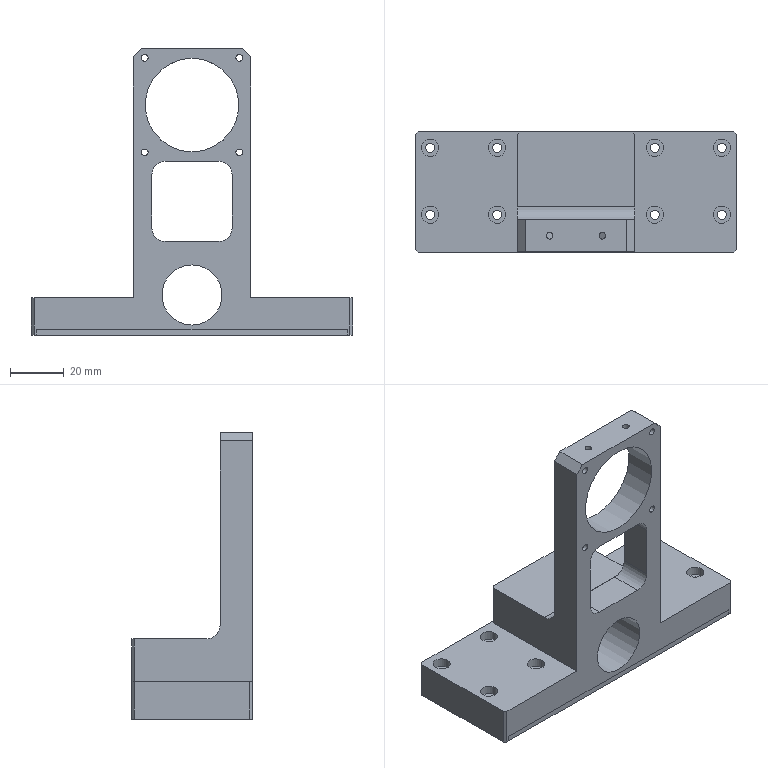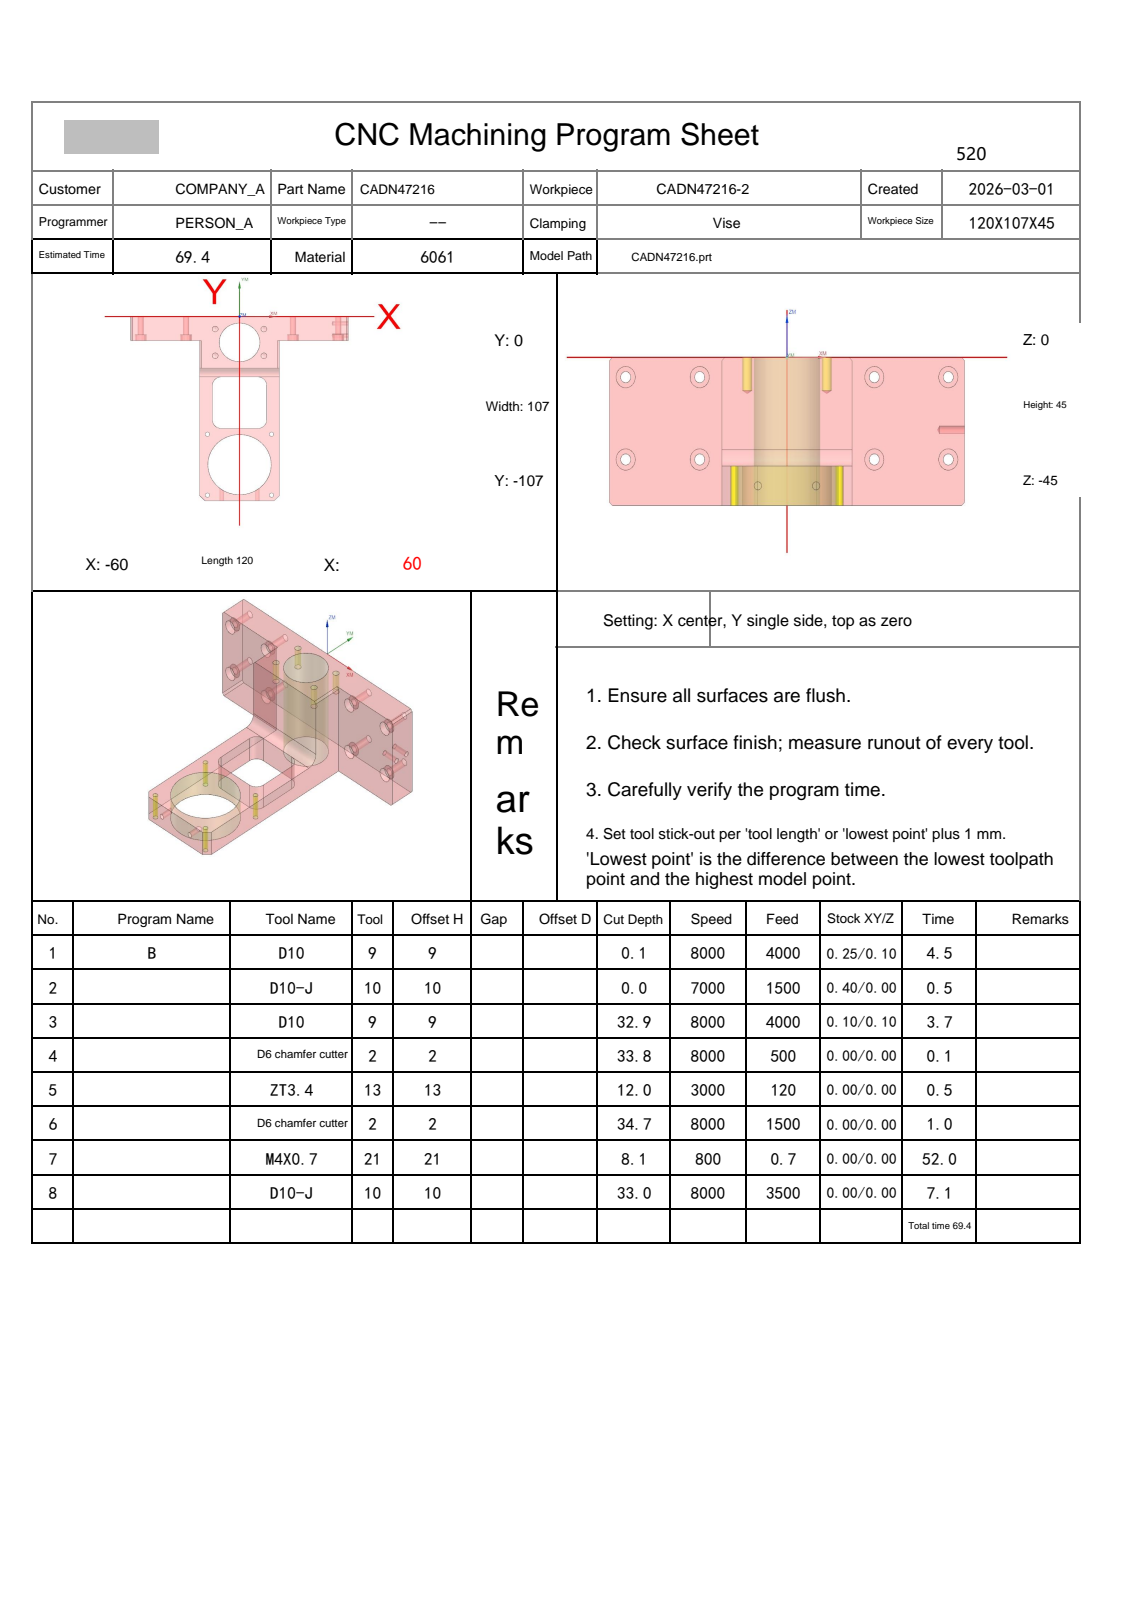NC program | NX | posted by the shop | part box 120 x 45 x 107 mm
Lines 1 to 768 of 8568:
%
O0001
(Machine time: 117.01 MIN)
(===Total Tool:5===)
(T9=D10     D=10.  R=0.   D-  H09 Z=-32.9 )
(T10=D10-J  D=10.  R=0.   D-  H10 Z=-33.  )
(T2=D6 chamfer cutter   D=6.   R=0.   D-  H02 Z=-34.75)
(T13=ZT3.4  D=3.4  DR_a=118 D-  H13 Z=-12.  )
(T21=M4X0.7 D=3.3  DR_a=180 D-  H21 Z=-8.1  )
G80 G90 G17 G49 G40
G91 G28 Z0
M01
N1 T09 M06
(D10  D=10. R=0. H=09 ce=0.25 di=0.10)
G00 G90 G54 X1.031 Y-119.091 M03 S8000
G43 H09 Z50.
M08
Z2.1
G01 X1.013 Y-118.992 Z1.476 F4000.
X.995 Y-118.894 Z1.228
X.977 Y-118.796 Z1.046
X.959 Y-118.697 Z.9
X.941 Y-118.599 Z.777
X.924 Y-118.5 Z.672
X.906 Y-118.402 Z.58
X.888 Y-118.304 Z.5
X.87 Y-118.205 Z.43
X.852 Y-118.107 Z.368
X.834 Y-118.009 Z.314
X.816 Y-117.91 Z.267
X.798 Y-117.812 Z.227
X.78 Y-117.713 Z.192
X.762 Y-117.615 Z.164
X.744 Y-117.517 Z.14
X.726 Y-117.418 Z.123
X.708 Y-117.32 Z.11
X.69 Y-117.222 Z.103
X.672 Y-117.123 Z.1
X.261 Y-114.872
G03 X-.031 Y-114.501 I-.503 J-.096
X-3.273 Y-113.892 I-3.513 J-9.76
X-11.635 Y-113.683 I-8.361 J-167.731
X-13.502 Y-113.694 I0.0 J-167.939
G01 X-60.698 Y-113.668
G02 X-65.816 Y-110.311 I.413 J6.208
X-67.398 Y-104.569 I12.799 J6.617
X-67.693 Y-96.578 I108.326 J7.991
X-67.683 Y-95.137 I108.62 J0.0
G01 X-67.668 Y-.345
G02 X-64.539 Y4.661 I6.122 J-.346
X-58.831 Y6.367 I6.686 J-11.968
X-50.974 Y6.692 I7.857 J-94.762
X-49.64 Y6.683 I0.0 J-95.087
G01 X60.716 Y6.666
G02 X65.706 Y3.458 I-.428 J-6.15
X67.374 Y-2.257 I-12.234 J-6.671
X67.701 Y-10.755 I-110.346 J-8.498
X67.685 Y-12.648 I-110.673 J0.0
G01 X67.664 Y-106.719
G02 X64.569 Y-111.639 I-6.109 J.409
X58.872 Y-113.362 I-6.688 J11.83
X51.057 Y-113.692 I-7.815 J92.457
X49.761 Y-113.683 I0.0 J92.787
G01 X2.742 Y-113.673
G03 X-4.124 Y-113.085 I-38.442 J-408.284
X-15.536 Y-112.878 I-11.412 J-314.384
X-18.539 Y-112.892 I0.0 J-314.591
G01 X-58.519 Y-112.871
G02 X-64.635 Y-108.899 I.605 J7.626
X-66.497 Y-102.658 I13.944 J7.559
X-66.892 Y-93.877 I97.4 J8.781
X-66.88 Y-92.35 I97.795 J0.0
G01 X-66.869 Y-2.505
G02 X-62.825 Y3.667 I7.656 J-.606
X-56.654 Y5.497 I7.53 J-14.076
X-48.188 Y5.887 I8.466 J-91.573
X-46.987 Y5.88 I0.0 J-91.963
G01 X58.556 Y5.867
G02 X64.614 Y1.908 I-.672 J-7.642
X66.482 Y-4.248 I-13.777 J-7.543
X66.886 Y-12.76 I-89.496 J-8.512
X66.877 Y-13.995 I-89.9 J0.0
G01 X66.87 Y-104.479
G02 X62.899 Y-110.622 I-7.642 J.584
X56.654 Y-112.497 I-7.58 J13.916
X48.387 Y-112.883 I-8.268 J88.324
X47.387 Y-112.877 I0.0 J88.71
G01 X4.367 Y-112.87
G02 X-4.415 Y-112.297 I59.52 J980.107
G03 X-16.402 Y-112.086 I-11.987 J-339.831
X-18.539 Y-112.093 I0.0 J-340.043
G01 X-56.518 Y-112.067
G02 X-63.736 Y-107.414 I.499 J8.699
X-65.657 Y-100.854 I15.568 J8.12
X-66.081 Y-91.909 I94.094 J8.945
X-66.075 Y-90.788 I94.518 J0.0
G01 X-66.071 Y-4.648
G02 X-61.215 Y2.84 I8.769 J-.367
X-54.546 Y4.693 I8.128 J-16.322
X-45.235 Y5.092 I9.311 J-108.369
X-43.758 Y5.082 I0.0 J-108.768
G01 X56.382 Y5.071
G02 X63.812 Y.261 I-.399 J-8.759
X65.674 Y-6.321 I-16.089 J-8.108
X66.091 Y-15.663 I-104.663 J-9.342
X66.08 Y-17.188 I-105.079 J0.0
G01 X66.072 Y-102.319
G02 X61.311 Y-109.787 I-8.749 J.326
X54.738 Y-111.67 I-8.11 J15.892
X45.886 Y-112.083 I-8.852 J94.835
X44.831 Y-112.077 I0.0 J95.248
G01 X5.892 Y-112.074
G02 X-4.561 Y-111.51 I22.142 J507.407
G03 X-18.122 Y-111.283 I-13.562 J-405.052
X-21.019 Y-111.293 I0.0 J-405.279
G01 X-54.519 Y-111.272
G02 X-63.058 Y-105.712 I.19 J9.628
X-64.884 Y-98.788 I18.235 J8.512
X-65.291 Y-88.985 I117.675 J9.803
X-65.28 Y-87.36 I118.083 J0.0
G01 X-65.264 Y-6.42
G02 X-59.794 Y2.013 I9.608 J-.242
X-52.871 Y3.874 I8.541 J-17.958
X-43.42 Y4.286 I9.451 J-108.294
X-42.163 Y4.279 I0.0 J-108.706
G01 X54.456 Y4.271
G02 X62.982 Y-1.156 I-.129 J-9.612
X64.864 Y-8.064 I-17.755 J-8.549
X65.283 Y-17.514 I-106.437 J-9.451
X65.275 Y-18.771 I-106.855 J0.0
G01 X65.27 Y-100.431
G02 X59.712 Y-109.053 I-9.642 J.113
X52.787 Y-110.884 I-8.531 J18.254
X42.903 Y-111.295 I-9.884 J118.498
X41.199 Y-111.283 I0.0 J118.909
G01 X6.739 Y-111.268
G02 X-4.786 Y-110.713 I22.344 J584.718
G03 X-18.776 Y-110.487 I-13.99 J-432.646
X-21.099 Y-110.493 I0.0 J-432.872
G01 X-52.839 Y-110.469
X-52.842
G02 X-62.185 Y-104.494 I0.0 J10.292
X-64.087 Y-97.085 I19.6 J8.982
X-64.486 Y-87.171 I122.962 J9.913
X-64.478 Y-85.736 I123.361 J0.0
G01 X-64.463 Y-8.156
G02 X-58.489 Y1.184 I10.291 J-.002
X-51.012 Y3.096 I9.028 J-19.733
X-41.101 Y3.488 I9.911 J-124.922
X-39.663 Y3.48 I0.0 J-125.314
G01 X52.797 Y3.467
X52.81
G02 X62.264 Y-2.679 I0.0 J-10.344
X64.096 Y-10.017 I-20.173 J-8.935
X64.485 Y-19.894 I-125.047 J-9.877
X64.477 Y-21.286 I-125.436 J0.0
G01 X64.462 Y-98.866
G02 X58.401 Y-108.226 I-10.313 J.035
X50.992 Y-110.098 I-8.975 J19.93
X41.129 Y-110.488 I-9.863 J124.38
X39.723 Y-110.48 I0.0 J124.771
G01 X7.743 Y-110.468
G02 X-5.171 Y-109.909 I20.139 J614.696
G03 X-20.354 Y-109.684 I-15.183 J-513.896
X-23.419 Y-109.694 I0.0 J-514.12
G01 X-51.239 Y-109.668
X-51.336 Y-109.669
G02 X-58.11 Y-107.406 I0.0 J11.271
X-62.307 Y-100.822 I8.301 J9.92
X-63.507 Y-92.529 I33.918 J9.144
X-63.706 Y-80.068 I390.427 J12.462
X-63.687 Y-76.212 I390.626 J0.0
G01 X-63.667 Y-9.912
X-63.669 Y-9.741
G02 X-61.686 Y-3.272 I11.544 J0.0
X-55.188 Y1.191 I9.98 J-7.567
X-47.152 Y2.475 I9.086 J-31.069
X-36.119 Y2.699 I11.033 J-271.555
X-33.635 Y2.688 I0.0 J-271.779
G01 X51.145 Y2.668
X51.283 Y2.669
G02 X57.837 Y.604 I0.0 J-11.438
X62.202 Y-5.858 I-7.763 J-9.948
X63.476 Y-13.898 I-31.281 J-9.077
X63.697 Y-24.945 I-275.857 J-11.047
X63.686 Y-27.415 I-276.078 J0.0
G01 X63.665 Y-97.155
X63.666 Y-97.29
G02 X61.551 Y-103.911 I-11.421 J0.0
X55.107 Y-108.215 I-9.919 J7.874
X46.747 Y-109.498 I-9.229 J32.264
X34.048 Y-109.711 I-12.699 J378.06
X30.03 Y-109.69 I0.0 J378.273
G01 X8.45 Y-109.665
G02 X-5.875 Y-109.093 I24.331 J788.851
G03 X-21.367 Y-108.886 I-15.492 J-581.127
X-24.299 Y-108.894 I0.0 J-581.334
G01 X-49.559 Y-108.873
G02 X-49.762 Y-108.875 I-.204 J12.906
X-55.863 Y-107.342 I0.0 J12.907
X-61.072 Y-100.838 I6.368 J10.437
X-62.612 Y-92.61 I27.924 J9.486
X-62.904 Y-80.847 I237.378 J11.762
X-62.885 Y-77.895 I237.669 J0.0
G01 X-62.862 Y-11.275
Y-11.146
G02 X-61.083 Y-4.72 I12.493 J0.0
X-54.743 Y.105 I10.289 J-6.941
X-46.429 Y1.626 I9.506 J-28.48
X-34.755 Y1.905 I11.674 J-244.361
X-31.874 Y1.888 I0.0 J-244.639
G01 X49.706 Y1.864
X49.843 Y1.865
G02 X56.262 Y.091 I0.0 J-12.498
X61.152 Y-6.394 I-6.979 J-10.349
X62.634 Y-14.719 I-29.198 J-9.49
X62.901 Y-26.357 I-253.031 J-11.638
X62.885 Y-29.195 I-253.299 J0.0
G01 X62.866 Y-95.575
X62.867 Y-95.772
G02 X61.286 Y-101.947 I-12.848 J0.0
X54.911 Y-107.041 I-10.388 J6.463
X46.848 Y-108.597 I-9.417 J27.144
X35.818 Y-108.898 I-11.03 J201.353
X33.574 Y-108.886 I0.0 J201.655
G01 X9.274 Y-108.866
G02 X-6.187 Y-108.29 I22.645 J816.699
G03 X-21.654 Y-108.091 I-15.467 J-600.289
X-23.579 Y-108.094 I0.0 J-600.488
G01 X-48.119 Y-108.073
G02 X-48.341 Y-108.074 I-.222 J14.228
X-54.326 Y-106.755 I0.0 J14.23
X-59.997 Y-100.34 I5.709 J10.762
X-61.74 Y-92.155 I25.544 J9.715
X-62.089 Y-81.354 I166.859 J10.802
X-62.08 Y-79.603 I167.208 J0.0
G01 X-62.068 Y-12.983
G02 X-62.071 Y-12.706 I14.437 J.278
X-60.793 Y-6.766 I14.439 J0.0
X-54.416 Y-1.036 I10.768 J-5.571
X-46.319 Y.726 I9.702 J-25.089
X-35.379 Y1.093 I10.941 J-163.267
X-33.528 Y1.082 I0.0 J-163.633
G01 X47.972 Y1.072
G02 X48.254 Y1.074 I.282 J-14.641
X54.121 Y-.152 I0.0 J-14.644
X59.999 Y-6.676 I-5.47 J-10.838
X61.739 Y-14.86 I-25.577 J-9.716
X62.089 Y-25.715 I-168.326 J-10.855
X62.08 Y-27.492 I-168.675 J0.0
G01 X62.069 Y-93.952
G02 X62.073 Y-94.259 I-14.606 J-.307
X60.821 Y-100.175 I-14.609 J0.0
X54.447 Y-105.95 I-10.777 J5.491
X46.512 Y-107.709 I-9.633 J24.667
X35.382 Y-108.095 I-11.13 J160.442
X33.402 Y-108.083 I0.0 J160.828
G01 X9.502 Y-108.059
G02 X-6.184 Y-107.497 I24.541 J904.536
G03 X-22.23 Y-107.291 I-16.046 J-625.487
X-24.299 Y-107.295 I0.0 J-625.693
G01 X-46.919 Y-107.267
X-47.099 Y-107.268
G02 X-53.357 Y-105.882 I0.0 J14.823
X-59.157 Y-99.296 I5.874 J11.02
X-60.929 Y-90.954 I26.24 J9.934
X-61.298 Y-79.194 I187.137 J11.76
X-61.282 Y-76.722 I187.506 J0.0
G01 X-61.265 Y-14.262
G02 X-61.267 Y-14.006 I15.388 J.256
X-60.026 Y-7.952 I15.39 J0.0
X-53.418 Y-1.896 I11.103 J-5.482
X-45.089 Y-.081 I9.956 J-25.682
X-34.093 Y.29 I10.996 J-162.688
X-32.377 Y.281 I0.0 J-163.06
G01 X46.723 Y.267
G02 X46.987 Y.27 I.264 J-15.401
X53.036 Y-.968 I0.0 J-15.404
X59.102 Y-7.583 I-5.469 J-11.104
X60.902 Y-15.754 I-25.38 J-9.877
X61.288 Y-26.851 I-159.643 J-11.098
X61.278 Y-28.624 I-160.028 J0.0
G01 X61.268 Y-92.604
G02 X61.271 Y-92.905 I-15.917 J-.301
X60.147 Y-98.781 I-15.92 J0.0
X53.477 Y-105.079 I-11.173 J5.15
X45.148 Y-106.914 I-9.976 J25.468
X34.102 Y-107.29 I-11.046 J161.959
X32.357 Y-107.281 I0.0 J162.336
G01 X10.297 Y-107.261
G02 X-6.735 Y-106.686 I24.309 J973.038
G03 X-22.948 Y-106.493 I-16.212 J-680.389
X-24.619 Y-106.495 I0.0 J-680.582
G01 X-45.399 Y-106.472
G02 X-45.667 Y-106.474 I-.268 J16.745
X-51.662 Y-105.365 I0.0 J16.747
X-58.207 Y-98.548 I5.104 J11.451
X-60.066 Y-90.388 I25.211 J10.037
X-60.479 Y-79.549 I142.281 J10.839
X-60.473 Y-78.319 I142.694 J0.0
G01 X-60.465 Y-15.619
G02 X-60.468 Y-15.327 I16.675 J.292
X-59.333 Y-9.281 I16.678 J0.0
X-52.781 Y-2.897 I11.356 J-5.101
X-44.483 Y-.942 I10.155 J-24.516
X-33.543 Y-.518 I10.94 J-140.745
X-32.174 Y-.524 I0.0 J-141.169
G01 X45.486 Y-.536
G02 X45.721 Y-.534 I.235 J-16.447
X51.741 Y-1.675 I0.0 J-16.449
X58.209 Y-8.466 I-5.185 J-11.414
X60.089 Y-16.864 I-25.618 J-10.143
X60.492 Y-28.509 I-167.795 J-11.645
X60.479 Y-30.615 I-168.198 J0.0
G01 X60.46 Y-91.554
G02 X60.462 Y-91.776 I-16.073 J-.222
X59.198 Y-98.024 I-16.074 J0.0
X52.512 Y-104.22 I-11.333 J5.523
X44.192 Y-106.086 I-10.1 J25.552
X32.957 Y-106.489 I-11.235 J156.651
X31.242 Y-106.479 I0.0 J157.054
G01 X11.182 Y-106.464
G02 X-5.783 Y-105.92 I16.054 J765.142
G03 X-22.839 Y-105.694 I-17.056 J-644.398
X-24.219 Y-105.695 I0.0 J-644.624
G01 X-44.359 Y-105.666
X-44.555 Y-105.667
G02 X-50.77 Y-104.49 I0.0 J17.
X-57.363 Y-97.578 I5.289 J11.644
X-59.272 Y-89.107 I25.924 J10.294
X-59.689 Y-77.465 I162.418 J11.641
X-59.677 Y-75.517 I162.835 J0.0
G01 X-59.666 Y-16.977
G02 X-59.669 Y-16.646 I18.207 J.332
X-58.641 Y-10.615 I18.21 J0.0
X-51.92 Y-3.791 I11.663 J-4.765
X-43.717 Y-1.787 I10.257 J-24.191
X-32.458 Y-1.318 I11.259 J-135.067
X-31.01 Y-1.326 I0.0 J-135.535
G01 X44.25 Y-1.337
G02 X44.484 Y-1.336 I.234 J-17.436
X50.597 Y-2.442 I0.0 J-17.437
X57.319 Y-9.327 I-5.066 J-11.67
X59.239 Y-17.554 I-25.184 J-10.215
X59.678 Y-28.711 I-141.276 J-11.157
X59.672 Y-30.022 I-141.715 J0.0
G01 X59.666 Y-90.002
G02 X59.669 Y-90.352 I-18.164 J-.35
X58.618 Y-96.442 I-18.167 J0.0
X51.945 Y-103.198 I-11.639 J4.823
X43.741 Y-105.211 I-10.255 J24.074
X32.458 Y-105.682 I-11.282 J134.923
X31.034 Y-105.674 I0.0 J135.394
G01 X12.014 Y-105.666
G02 X-6.255 Y-105.11 I15.719 J816.109
G03 X-23.899 Y-104.891 I-17.644 J-713.502
X-26.379 Y-104.896 I0.0 J-713.72
G02 X-32.415 Y-104.917 I-6.035 J842.947
X-43.878 Y-104.839 I0.0 J842.968
X-50.672 Y-103.242 I.091 J15.637
X-56.616 Y-96.407 I6.435 J11.597
X-58.488 Y-87.759 I27.35 J10.447
X-58.886 Y-76.191 I167.885 J11.567
X-58.876 Y-74.408 I168.283 J0.0
G01 X-58.864 Y-18.188
G02 X-58.867 Y-17.854 I19.225 J.334
X-57.868 Y-11.737 I19.228 J0.0
X-51.029 Y-4.661 I11.891 J-4.648
X-42.594 Y-2.592 I10.484 J-24.514
X-31.246 Y-2.12 I11.348 J-136.409
X-29.888 Y-2.127 I0.0 J-136.88
G01 X42.732 Y-2.132
G02 X43.091 Y-2.129 I.359 J-19.631
X49.113 Y-3.075 I0.0 J-19.634
X56.405 Y-10.117 I-4.531 J-11.989
X58.43 Y-18.643 I-25.2 J-10.489
X58.876 Y-29.85 I-140.649 J-11.207
X58.87 Y-31.111 I-141.095 J0.0
G01 X58.865 Y-88.771
G02 X58.868 Y-89.121 I-19.376 J-.351
X57.882 Y-95.224 I-19.38 J0.0
X50.93 Y-102.386 I-11.931 J4.625
X42.648 Y-104.403 I-10.391 J24.658
X31.253 Y-104.88 I-11.395 J135.764
X29.862 Y-104.873 I0.0 J136.241
X22.378 Y-104.91 I-7.484 J753.01
X5.084 Y-104.712 I0.0 J753.047
G03 X-24.018 Y-104.087 I-29.102 J-677.044
X-27.579 Y-104.096 I0.0 J-677.669
G02 X-32.634 Y-104.116 I-5.055 J623.468
X-42.838 Y-104.033 I0.0 J623.489
X-49.64 Y-102.455 I.142 J16.063
X-55.795 Y-95.428 I6.408 J11.821
X-57.665 Y-86.859 I27.56 J10.505
X-58.086 Y-75.088 I164.617 J11.771
X-58.076 Y-73.269 I165.037 J0.0
G01 X-58.065 Y-19.449
G02 X-58.067 Y-19.107 I20.85 J.342
X-57.171 Y-13.058 I20.852 J0.0
X-50.067 Y-5.487 I12.204 J-4.332
X-41.558 Y-3.402 I10.612 J-24.897
X-30.022 Y-2.921 I11.536 J-138.016
X-28.612 Y-2.928 I0.0 J-138.497
G01 X41.768 Y-2.938
G02 X42.07 Y-2.936 I.302 J-19.48
X48.371 Y-3.983 I0.0 J-19.482
X55.559 Y-11.036 I-4.819 J-12.101
X57.607 Y-19.556 I-25.318 J-10.591
X58.075 Y-30.985 I-139.215 J-11.429
X58.07 Y-32.262 I-139.683 J0.0
G01 X58.063 Y-87.602
G02 X58.066 Y-87.939 I-20.493 J-.336
X57.129 Y-94.066 I-20.496 J0.0
X49.904 Y-101.588 I-12.21 J4.497
X41.458 Y-103.608 I-10.543 J25.419
X30.012 Y-104.079 I-11.446 J139.033
X28.671 Y-104.072 I0.0 J139.503
X21.702 Y-104.11 I-6.969 J642.078
X-5.062 Y-103.552 I0.0 J642.116
G03 X-24.079 Y-103.293 I-19.017 J-699.356
X-26.22 Y-103.297 I0.0 J-699.615
G02 X-31.32 Y-103.317 I-5.101 J633.165
X-41.718 Y-103.232 I0.0 J633.185
X-48.538 Y-101.713 I.145 J16.724
X-54.915 Y-94.609 I6.251 J12.025
X-56.851 Y-85.894 I27.481 J10.676
X-57.286 Y-73.93 I164.33 J11.964
X-57.275 Y-72.065 I164.765 J0.0
G01 X-57.267 Y-20.805
G02 X-57.272 Y-20.36 I22.449 J.446
X-56.401 Y-14.168 I22.454 J0.0
X-49.289 Y-6.391 I12.375 J-4.176
X-40.954 Y-4.257 I10.66 J-24.302
X-29.4 Y-3.728 I11.554 J-125.689
X-28.25 Y-3.733 I0.0 J-126.219
G01 X40.21 Y-3.731
G02 X40.623 Y-3.727 I.413 J-22.729
X46.694 Y-4.553 I0.0 J-22.733
X54.621 Y-11.738 I-4.045 J-12.428
X56.752 Y-20.153 I-24.48 J-10.678
X57.269 Y-31.618 I-126.939 J-11.465
X57.264 Y-32.697 I-127.455 J0.0
G01 X57.267 Y-86.197
G02 X57.271 Y-86.623 I-22.733 J-.426
X56.449 Y-92.682 I-22.737 J0.0
X49.142 Y-100.679 I-12.451 J4.04
X40.632 Y-102.778 I-10.702 J25.082
X28.861 Y-103.28 I-11.771 J137.902
X27.366 Y-103.272 I0.0 J138.404
X21.682 Y-103.296 I-5.684 J673.985
X-6.011 Y-102.727 I0.0 J674.009
G03 X-24.901 Y-102.493 I-18.889 J-764.912
X-27.18 Y-102.497 I0.0 J-765.146
G02 X-31.56 Y-102.519 I-4.38 J424.484
X-40.918 Y-102.416 I0.0 J424.507
X-47.865 Y-100.76 I.272 J16.535
X-54.107 Y-93.638 I6.613 J12.092
X-56.047 Y-84.839 I28.042 J10.797
X-56.485 Y-72.727 I167.276 J12.112
X-56.474 Y-70.85 I167.714 J0.0
G01 X-56.459 Y-21.59
G02 X-56.462 Y-21.26 I21.733 J.33
X-55.506 Y-14.886 I21.736 J0.0
X-48.343 Y-7.209 I12.491 J-4.474
X-39.771 Y-5.046 I10.832 J-24.863
X-28.159 Y-4.528 I11.612 J-129.932
X-26.986 Y-4.533 I0.0 J-130.45
G01 X39.473 Y-4.54
G02 X39.763 Y-4.538 I.289 J-21.616
X46.098 Y-5.487 I0.0 J-21.618
X53.77 Y-12.613 I-4.44 J-12.473
X55.938 Y-21.105 I-24.651 J-10.816
X56.47 Y-32.821 I-128.609 J-11.715
X56.465 Y-34.049 I-129.141 J0.0
G01 X56.458 Y-85.469
G02 X56.46 Y-85.787 I-21.322 J-.319
X55.459 Y-92.244 I-21.324 J0.0
X48.244 Y-99.839 I-12.467 J4.62
X39.9 Y-101.939 I-10.718 J24.946
X28.172 Y-102.473 I-11.728 J128.635
X26.956 Y-102.467 I0.0 J129.168
X21.651 Y-102.488 I-5.305 J685.365
X-6.01 Y-101.929 I0.0 J685.385
G03 X-28.656 Y-101.672 I-22.646 J-996.432
X-35.479 Y-101.695 I0.0 J-996.689
G02 X-36.72 Y-101.712 I-1.241 J45.813
X-42.662 Y-101.326 I0.0 J45.829
X-52.939 Y-93.49 I1.973 J13.245
X-55.119 Y-85.004 I24.744 J10.882
X-55.666 Y-73.289 I125.227 J11.715
X-55.662 Y-72.222 I125.774 J0.0
G01 X-55.667 Y-23.122
G02 X-55.671 Y-22.649 I24.871 J.472
X-54.871 Y-16.391 I24.876 J0.0
X-47.395 Y-8.019 I12.814 J-3.919
X-38.814 Y-5.858 I10.906 J-25.188
X-26.929 Y-5.326 I11.885 J-132.596
X-25.63 Y-5.333 I0.0 J-133.128
G01 X37.87 Y-5.331
G02 X38.342 Y-5.327 I.472 J-24.945
X44.601 Y-6.125 I0.0 J-24.949
X52.994 Y-13.633 I-3.915 J-12.821
X55.143 Y-22.212 I-25.335 J-10.906
X55.671 Y-34.083 I-133.215 J-11.871
X55.665 Y-35.316 I-133.743 J0.0
G01 X55.662 Y-84.096
G02 X55.666 Y-84.478 I-23.911 J-.382
X54.831 Y-90.741 I-23.914 J0.0
X47.518 Y-98.924 I-12.734 J4.02
X39.191 Y-101.099 I-10.83 J24.443
X27.552 Y-101.664 I-11.639 J119.449
X26.65 Y-101.661 I0.0 J120.014
X21.206 Y-101.684 I-5.444 J658.59
X-5.135 Y-101.157 I0.0 J658.613
G03 X-28.761 Y-100.873 I-23.626 J-985.296
X-35.079 Y-100.894 I0.0 J-985.579
G02 X-36.135 Y-100.908 I-1.056 J38.083
X-42.33 Y-100.401 I0.0 J38.098
X-52.053 Y-92.714 I2.565 J13.236
X-54.316 Y-83.994 I24.827 J11.095
X-54.868 Y-72.052 I128.807 J11.942
X-54.863 Y-70.892 I129.359 J0.0
G01 X-54.861 Y-23.952
G02 X-54.864 Y-23.578 I24.556 J.374
X-54.028 Y-17.226 I24.558 J0.0
X-46.603 Y-8.896 I12.908 J-4.032
X-38.12 Y-6.698 I10.964 J-24.842
X-26.284 Y-6.134 I11.836 J-123.883
X-25.258 Y-6.138 I0.0 J-124.447
G01 X36.961 Y-6.135
G02 X37.376 Y-6.132 I.415 J-24.827
X43.768 Y-6.968 I0.0 J-24.83
X52.145 Y-14.487 I-4.025 J-12.911
X54.322 Y-23.064 I-25.294 J-10.983
X54.86 Y-34.655 I-124.378 J-11.591
X54.858 Y-35.447 I-124.917 J0.0
G01 X54.861 Y-83.027
G02 X54.864 Y-83.408 I-24.659 J-.381
X54.034 Y-89.754 I-24.662 J0.0
X46.708 Y-98.054 I-12.864 J3.971
X38.231 Y-100.289 I-10.989 J24.488
X26.315 Y-100.867 I-11.916 J122.458
X25.21 Y-100.863 I0.0 J123.037
X21.178 Y-100.875 I-4.033 J675.673
X-5.451 Y-100.35 I0.0 J675.685
G03 X-28.933 Y-100.073 I-23.482 J-996.269
X-34.699 Y-100.09 I0.0 J-996.546
G02 X-35.515 Y-100.1 I-.816 J33.478
X-41.781 Y-99.508 I0.0 J33.488
X-51.282 Y-91.71 I2.968 J13.302
X-53.523 Y-82.908 I25.497 J11.177
X-54.072 Y-70.667 I136.083 J12.242
X-54.065 Y-69.245 I136.632 J0.0
G01 X-54.061 Y-25.025
G02 X-54.063 Y-24.665 I25.613 J.36
X-53.258 Y-18.293 I25.616 J0.0
X-45.614 Y-9.676 I13.1 J-3.922
X-36.967 Y-7.483 I11.087 J-25.567
X-24.956 Y-6.931 I12.011 J-130.377
X-23.784 Y-6.936 I0.0 J-130.929
G01 X35.956 Y-6.937
G02 X36.343 Y-6.934 I.387 J-25.46
X42.765 Y-7.757 I0.0 J-25.463
X51.303 Y-15.341 I-3.969 J-13.066
X53.501 Y-23.905 I-25.283 J-11.053
X54.067 Y-35.969 I-128.191 J-12.064
X54.062 Y-37.167 I-128.758 J0.0
G01 X54.061 Y-81.947
G02 X54.064 Y-82.33 I-25.59 J-.383
X53.244 Y-88.757 I-25.593 J0.0
X45.637 Y-97.315 I-13.068 J3.957
X36.987 Y-99.515 I-11.089 J25.487
X25.003 Y-100.069 I-11.984 J129.45
X23.804 Y-100.063 I0.0 J130.003
X21.489 Y-100.067 I-2.315 J711.326
X-5.926 Y-99.538 I0.0 J711.33
G03 X-28.44 Y-99.275 I-22.514 J-963.864
X-33.64 Y-99.289 I0.0 J-964.127
G02 X-34.455 Y-99.299 I-.815 J34.576
X-40.803 Y-98.711 I0.0 J34.586
X-50.489 Y-90.759 I2.945 J13.462
X-52.725 Y-81.877 I25.962 J11.258
X-53.267 Y-69.79 I134.52 J12.087
X-53.262 Y-68.613 I135.062 J0.0
G01 X-53.261 Y-26.153
G02 X-53.265 Y-25.724 I26.289 J.43
X-52.438 Y-19.183 I26.292 J0.0
X-44.759 Y-10.514 I13.2 J-3.956
X-36.114 Y-8.301 I11.154 J-25.582
X-24.213 Y-7.738 I11.901 J-125.396
X-23.332 Y-7.741 I0.0 J-125.959
G01 X34.807 Y-7.736
G02 X35.253 Y-7.732 I.445 J-26.507
X41.779 Y-8.548 I0.0 J-26.51
X50.465 Y-16.197 I-3.903 J-13.189
X52.701 Y-24.919 I-25.535 J-11.192
X53.27 Y-37.232 I-133.052 J-12.313
X53.263 Y-38.581 I-133.62 J0.0
G01 X53.261 Y-80.801
G02 X53.265 Y-81.227 I-26.844 J-.426
X52.474 Y-87.696 I-26.847 J0.0
X44.708 Y-96.511 I-13.239 J3.835
X35.821 Y-98.732 I-11.247 J26.105
X23.724 Y-99.27 I-12.097 J135.912
X22.397 Y-99.263 I0.0 J136.449
X21.22 Y-99.264 I-1.177 J686.612
X-4.812 Y-98.771 I0.0 J686.613
G03 X-28.734 Y-98.475 I-23.922 J-967.225
X-33.101 Y-98.485 I0.0 J-967.521
G02 X-33.724 Y-98.491 I-.623 J32.22
X-40.098 Y-97.854 I0.0 J32.226
X-49.693 Y-89.826 I3.169 J13.534
X-51.893 Y-81.164 I25.974 J11.209
X-52.463 Y-69.044 I128.651 J12.12
X-52.458 Y-67.982 I129.221 J0.0
G01 X-52.459 Y-27.122
G02 X-52.462 Y-26.708 I26.603 J.415
X-51.622 Y-20.074 I26.606 J0.0
X-43.827 Y-11.312 I13.313 J-3.995
X-35.02 Y-9.09 I11.266 J-26.09
X-22.954 Y-8.535 I12.066 J-130.969
X-21.917 Y-8.539 I0.0 J-131.524
G01 X33.823 Y-8.538
G02 X34.25 Y-8.534 I.427 J-26.976
X40.873 Y-9.36 I0.0 J-26.979
X49.623 Y-17.032 I-3.911 J-13.286
X51.873 Y-25.671 I-25.415 J-11.229
X52.463 Y-37.895 I-126.242 J-12.225
X52.458 Y-39.011 I-126.832 J0.0
G01 X52.464 Y-79.551
G02 X52.469 Y-80.081 I-28.409 J-.53
X51.69 Y-86.689 I-28.414 J0.0
X44.019 Y-95.598 I-13.335 J3.725
X35.309 Y-97.877 I-11.271 J25.295
X23.204 Y-98.462 I-12.105 J124.915
X22.048 Y-98.457 I0.0 J125.5
G01 X21.464
G02 X-5.367 Y-97.956 I0.0 J719.164
G03 X-28.612 Y-97.676 I-23.245 J-964.205
X-32.223 Y-97.683 I0.0 J-964.485
G02 X-32.808 Y-97.688 I-.585 J31.83
X-39.296 Y-97.02 I0.0 J31.835
X-48.832 Y-89.036 I3.28 J13.604
X-51.077 Y-80.313 I25.832 J11.301
X-51.662 Y-68.034 I128.588 J12.28
X-51.658 Y-66.972 I129.173 J0.0
G01 X-51.659 Y-28.192
G02 X-51.663 Y-27.766 I27.75 J.426
X-50.859 Y-21.138 I27.753 J0.0
X-43.27 Y-12.282 I13.386 J-3.793
X-34.496 Y-9.943 I11.38 J-25.063
X-22.483 Y-9.344 I12.013 J-120.001
X-21.716 Y-9.346 I0.0 J-120.601
G01 X31.704 Y-9.325
G02 X32.51 Y-9.315 I.807 J-35.029
X39.025 Y-9.926 I0.0 J-35.039
X48.833 Y-17.972 I-2.998 J-13.656
X51.078 Y-26.697 I-25.86 J-11.304
X51.658 Y-38.793 I-125.706 J-12.096
X51.655 Y-39.718 I-126.287 J0.0
G01 X51.659 Y-78.818
G02 X51.662 Y-79.252 I-27.529 J-.434
X50.835 Y-85.949 I-27.533 J0.0
X43.04 Y-94.828 I-13.419 J3.921
X34.166 Y-97.096 I-11.374 J26.002
X21.917 Y-97.664 I-12.248 J131.684
X20.424 Y-97.656 I0.0 J132.253
X-5.764 Y-97.147 I1.822 J768.446
G03 X-29.033 Y-96.875 I-23.269 J-993.129
X-31.584 Y-96.878 I0.0 J-993.402
G02 X-32.041 Y-96.882 I-.457 J30.155
X-38.649 Y-96.149 I0.0 J30.158
X-48.051 Y-88.085 I3.555 J13.657
X-50.266 Y-79.439 I26.126 J11.3
X-50.857 Y-67.268 I125.13 J12.171
X-50.854 Y-66.419 I125.72 J0.0
G01 X-50.864 Y-29.559
G02 X-50.869 Y-29.017 I30.752 J.542
X-50.151 Y-22.411 I30.756 J0.0
X-42.254 Y-13.031 I13.606 J-3.44
X-33.387 Y-10.727 I11.439 J-25.806
X-21.016 Y-10.135 I12.371 J-129.134
X-19.886 Y-10.14 I0.0 J-129.725
G01 X31.773 Y-10.139
G02 X32.189 Y-10.136 I.416 J-28.86
X38.833 Y-10.911 I0.0 J-28.863
X48.004 Y-18.821 I-3.706 J-13.57
X50.253 Y-27.456 I-25.764 J-11.319
X50.861 Y-39.877 I-126.499 J-12.42
X50.857 Y-40.956 I-127.107 J0.0
G01 X50.858 Y-77.816
G02 X50.862 Y-78.259 I-28.065 J-.443
X50.033 Y-85.029 I-28.069 J0.0
X42.408 Y-93.894 I-13.471 J3.875
X33.624 Y-96.245 I-11.432 J25.124
X21.342 Y-96.857 I-12.281 J123.011
X19.884 Y-96.848 I0.0 J123.622
X-6.479 Y-96.33 I3.01 J824.776
G03 X-28.649 Y-96.076 I-22.17 J-966.261
X-30.626 Y-96.078 I0.0 J-966.516
G02 X-31.11 Y-96.082 I-.484 J29.949
X-37.925 Y-95.296 I0.0 J29.953
X-47.14 Y-87.418 I3.704 J13.661
X-49.439 Y-78.709 I25.636 J11.424
X-50.052 Y-66.53 I120.585 J12.179
X-50.05 Y-65.77 I121.198 J0.0
G01 X-50.068 Y-30.91
G02 X-50.075 Y-30.219 I33.431 J.691
X-49.397 Y-23.517 I33.438 J0.0
X-41.2 Y-13.759 I13.81 J-3.28
X-32.394 Y-11.523 I11.427 J-26.533
X-20.29 Y-10.944 I12.104 J-126.249
X-19.533 Y-10.946 I0.0 J-126.828
G01 X29.967 Y-10.929
G02 X30.671 Y-10.922 I.703 J-34.904
X37.286 Y-11.554 I0.0 J-34.911
X47.172 Y-19.657 I-3.074 J-13.832
X49.485 Y-28.686 I-26.296 J-11.546
X50.056 Y-40.857 I-129.311 J-12.171
X50.054 Y-41.708 I-129.883 J0.0
G01 X50.059 Y-76.727
G02 X50.063 Y-77.193 I-29.443 J-.465
X49.278 Y-83.946 I-29.447 J0.0
X41.393 Y-93.149 I-13.647 J3.713
X32.607 Y-95.452 I-11.449 J25.762
X20.617 Y-96.046 I-11.99 J120.683
X19.347 Y-96.04 I0.0 J121.277
X-6.875 Y-95.522 I4.292 J882.56
G03 X-28.219 Y-95.279 I-21.344 J-936.403
X-29.589 Y-95.28 I0.0 J-936.647
G02 X-30.055 Y-95.284 I-.466 J31.442
X-36.815 Y-94.548 I0.0 J31.446
X-46.381 Y-86.435 I3.503 J13.827
X-48.672 Y-77.482 I26.505 J11.55
X-49.264 Y-64.837 I134.751 J12.645
X-49.258 Y-63.581 I135.343 J0.0
G01 X-49.263 Y-31.521
G02 X-49.268 Y-30.954 I31.547 J.567
X-48.523 Y-24.136 I31.552 J0.0
X-40.635 Y-14.717 I13.763 J-3.513
X-31.935 Y-12.382 I11.478 J-25.384
X-19.521 Y-11.744 I12.414 J-120.51
X-18.597 Y-11.747 I0.0 J-121.148
G01 X28.583 Y-11.726
G02 X29.428 Y-11.716 I.845 J-38.767
X36.069 Y-12.289 I0.0 J-38.777
X46.402 Y-20.615 I-2.778 J-14.023
X48.668 Y-29.494 I-26.549 J-11.506
X49.261 Y-42.032 I-132.289 J-12.538
X49.256 Y-43.155 I-132.882 J0.0
G01 X49.264 Y-75.375
G02 X49.269 Y-75.938 I-32.938 J-.563
X48.586 Y-82.608 I-32.943 J0.0
X40.508 Y-92.343 I-13.864 J3.285
X31.644 Y-94.653 I-11.52 J26.035
X19.449 Y-95.246 I-12.195 J125.215
X17.584 Y-95.232 I0.0 J125.808
X-5.92 Y-94.747 I6.601 J890.364
G03 X-28.901 Y-94.476 I-22.982 J-971.17
G01 X-28.952
G02 X-29.306 Y-94.478 I-.354 J29.909
X-36.17 Y-93.679 I0.0 J29.911
X-45.544 Y-85.622 I3.744 J13.837
X-47.837 Y-76.831 I26.183 J11.524
X-48.447 Y-64.715 I120.156 J12.116
X-48.445 Y-64.132 I120.765 J0.0